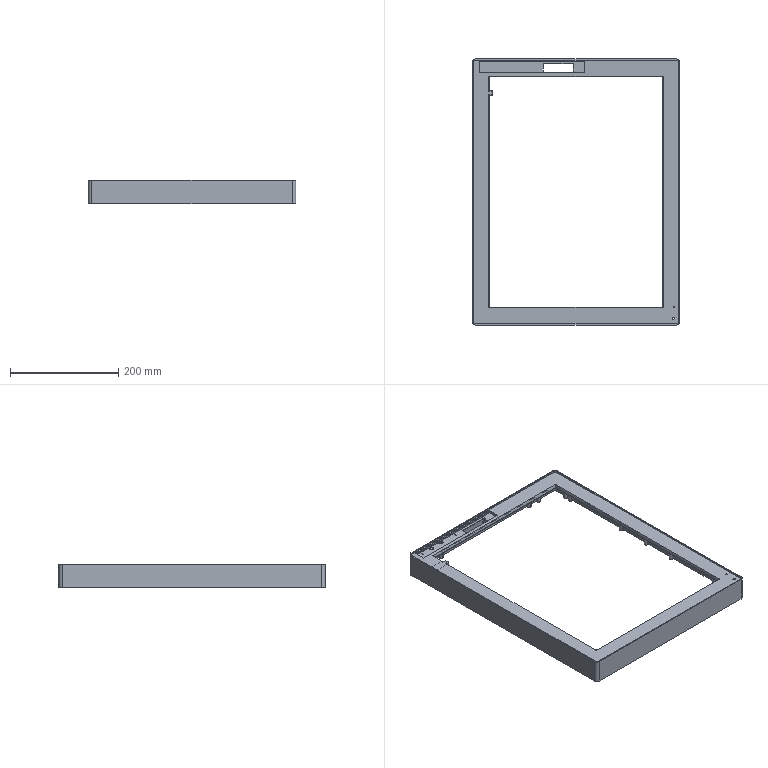Part | Creo | 1 solid | 1040 faces | box 383 x 491 x 44.1 mm | volume 408160 mm3 | plane 840 | cylinder 182 | cone 10 | torus 4 | spline 2 | sphere 2 | commonest cylinder face diameters 4 x46 8 x44 3 x33 10 x27 34.275 x5 1.2 x4